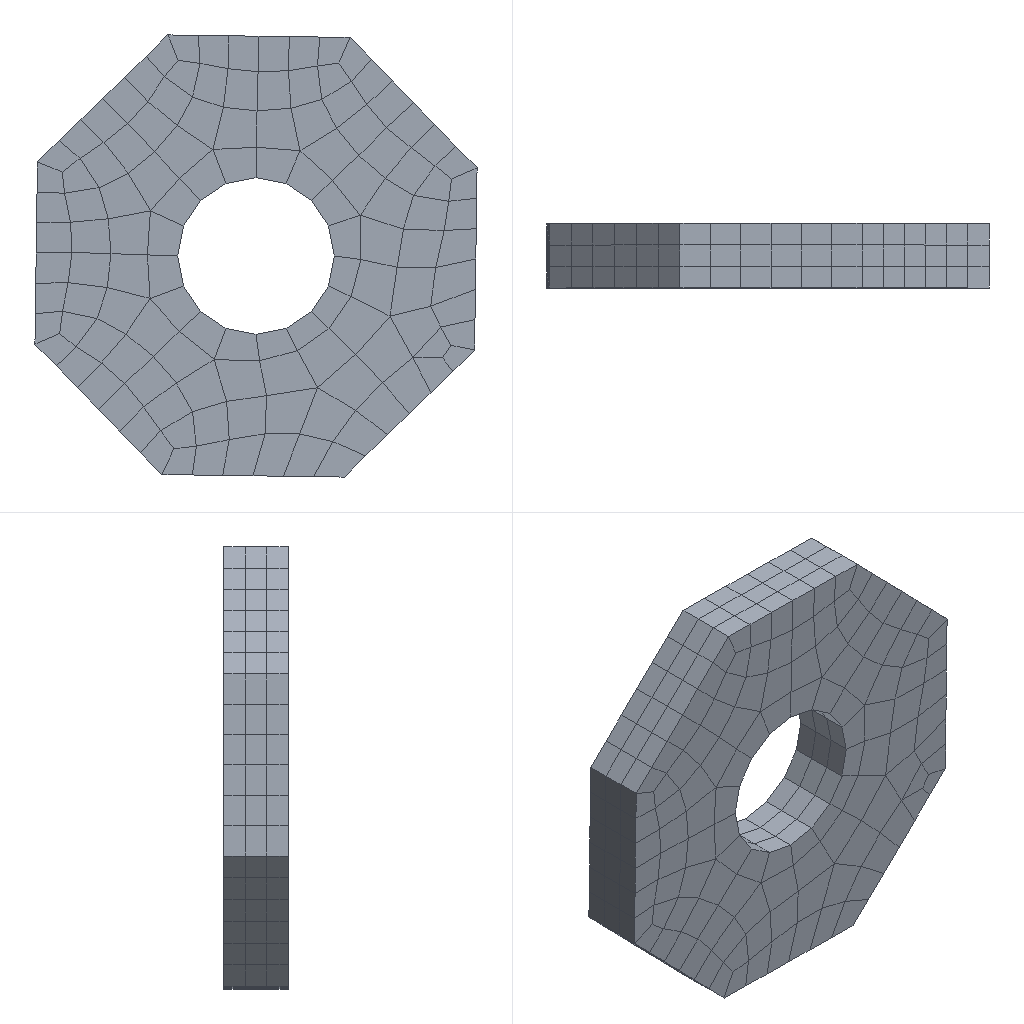Simulation study | ansys workbench
Ansys APDL input file, long lists of numbers shortened:
/batch
/config,noeldb,1     ! force off writing results to database
*get,_wallstrt,active,,time,wall
! ANSYS input file written by Workbench version 2022 R1
! File used for geometry attach: F:\ansys（分析文件汇总)\桥梁分析\平面.STEP
/title,__--____ (C5)
! ****** Begin Custom Load Command Snippet ******
/COM, ACT Extensions:
/COM,     LSDYNA, 2021.1
/COM,
! ****** End   Custom Load Command Snippet ******
*DIM,_wb_ProjectScratch_dir,string,248
_wb_ProjectScratch_dir(1) = 'F:\ansys（分析文件汇总)\桥梁分析\_ProjectScratch\ScrD469\'
*DIM,_wb_SolverFiles_dir,string,248
_wb_SolverFiles_dir(1) = 'F:\ansys（分析文件汇总)\桥梁分析\桥梁_files\dp0\SYS-2\MECH\'
*DIM,_wb_userfiles_dir,string,248
_wb_userfiles_dir(1) = 'F:\ansys（分析文件汇总)\桥梁分析\桥梁_files\user_files\'
/com,--- Data in consistent NMM units. See Solving Units in the help system for more information.
/units,MPA
/nopr
/wb,file,start              !  signify a WB generated input file
/prep7
! Turn off shape checking because checks already performed inside WB mesher.
! See help system for more information.
SHPP,OFF,,NOWARN
/nolist
etcon,set             ! allow ANSYS to choose best KEYOP's for 180x elements, resets any applicable keyopt to MAPDL defaults
/com,*********** Nodes for the whole assembly ***********
nblock,3,,2400
(1i9,3e20.9e3)
        1     1.551549580E+01     3.333333333E+00    -1.526301405E+01
! (2181 more lines like these left out)
-1
/wb,elem,start            !  set before creation of elements
/com,*********** Elements for Body 1 "__-FreeParts|__-__1" ***********
et,1,186
keyo,1,2,1          ! set full integration on SOLID186
eblock,19,solid,,366
(19i9)
        1        1        1        1        0        0        0        0       20        0        1        1       79       29       95      270      231      256      223
! (731 more lines like these left out)
-1
/wb,elem,end               !  done creating elements
/com,*********** Send User Defined Coordinate System(s) ***********
csys,0
toffst,273.15,  ! Temperature offset from absolute zero
/com,*********** Set Reference Temperature ***********
tref,22.
/wb,mat,start              !  starting to send materials
/com,*********** Send Materials ***********
Temperature = 'TEMP' ! Temperature
MP,DENS,1,7.85e-09,	! tonne mm^-3
MP,ALPX,1,1.2e-05,	! C^-1
MP,C,1,434000000,	! mm^2 s^-2 C^-1
MP,KXX,1,60.5,	! tonne mm s^-3 C^-1
MP,RSVX,1,0.00017,	! ohm mm
MP,EX,1,200000,	! tonne s^-2 mm^-1
MP,NUXY,1,0.3,
MP,MURX,1,10000,
/wb,mat,end                !  done sending materials
!************************* Model Summary ********************
!__-FreeParts|__-__1,	结构钢,	matid,	1
!************************* End Model Summary ********************
! get the diagonal of the bounding box. Needed later for other things
*get,_xmin,node,,mnloc,x
*get,_ymin,node,,mnloc,y
*get,_zmin,node,,mnloc,z
*get,_xmax,node,,mxloc,x
*get,_ymax,node,,mxloc,y
*get,_zmax,node,,mxloc,z
_ASMDIAG=(_xmax-_xmin)*(_xmax-_xmin)+(_ymax-_ymin)*(_ymax-_ymin)+(_zmax-_zmin)*(_zmax-_zmin)
_ASMDIAG=SQRT(_ASMDIAG)
/wb,contact,start          !  starting to send contact
/wb,contact,end            !  done creating contacts
/golist
/wb,load,start             !  starting to send loads
/com,*********** Fixed Supports ***********
CMBLOCK,_FIXEDSU,NODE,      430
(8i10)
       181       182       183       184       185       186       187       188
! (53 more lines like these left out)
cmsel,s,_FIXEDSU
d,all,all
nsel,all
/com,*********** Define Force Using Surface Effect Elements ***********
local,12,0,0.,0.,0.,0.,0.,0.
csys,0
et,2,154
eblock,10,,,48
(15i9)
      803        2        2        2       12      448      425      424      423     1865     1862     1860     1861
! (47 more lines like these left out)
-1
esel,s,type,,2
keyop,2,2,1                ! Apply load in local coordinate system
keyop,2,7,1                ! Use original area so load is constant in large deformation
esel,all
/gst,on,on
fini
*get,_numnode,node,0,count
*get,_numelem,elem,0,count
*get, _MAXELEMNUM, elem, 0, NUM, MAX
*get, _MAXNODENUM, node, 0, NUM, MAX
*get, _MAXELEMTYPE, etyp, 0, NUM, MAX
*get, _MAXREALCONST, real, 0, NUM, MAX
/go
/wb,load,end               !  done creating loads
/com,--- Number of total nodes = %_numnode%
/com,--- Number of contact elements = 48
/com,--- Number of spring elements = 0
/com,--- Number of bearing elements = 0
/com,--- Number of solid elements = 366
/com,--- Number of condensed parts = 0
/com,--- Number of total elements = %_numelem%
*get,_wallbsol,active,,time,wall
/com,****************************************************************************
/com,*************************    SOLUTION       ********************************
/com,****************************************************************************
/solu
antype,0                   ! static analysis
_thickRatio=  1     ! Ratio of thick parts in the model
eqsl,pcg,1e-8,,,,,,1
cntr,print,1               ! print out contact info and also make no initial contact an error
dmpoption,emat,no             ! Don't combine emat file for DANSYS
dmpoption,esav,no             ! Don't combine esav file for DANSYS
nldiag,cont,iter           ! print out contact info each equilibrium iteration
rescontrol,,none                 ! Do not keep any restart files
/com,****************************************************
/com,******************* SOLVE FOR LS 1 OF 1 ****************
esel,s,type,,2
nsle
sfe,all,1,pres,1,0.1216
sfe,all,2,pres,1,0.1216
sfe,all,3,pres,1,0.1216
nsel,all
esel,all
/nopr
/gopr
nsub,1,1,1
time,1.
outres,erase
outres,all,none
outres,nsol,all,
outres,rsol,all
outres,eangl,all
outres,etmp,all
outres,veng,all
outres,strs,all,
outres,epel,all,
outres,eppl,all,
outres,cont,all,
! *********** WB SOLVE COMMAND ***********
! check interactive state
*get,ANSINTER_,active,,int
*if,ANSINTER_,ne,0,then
/eof
*endif
solve
/com *************** Write FE CONNECTORS *********
CEWRITE,file,ce,,INTE
/com,****************************************************
/com,*************** FINISHED SOLVE FOR LS 1 *************
*get,_wallasol,active,,time,wall
/nopr
*get,_numnode,node,0,count
*get,_numelem,elem,0,count
*get, _MAXELEMNUM, elem, 0, NUM, MAX
*get, _MAXNODENUM, node, 0, NUM, MAX,,,INTERNAL
*get, _MAXELEMTYPE, etyp, 0, NUM, MAX
*get, _MAXREALCONST, real, 0, NUM, MAX
/gopr
*get,_PCGITER,active,,solu,cgiter
/post1
xmlo,ENCODING,ISO-8859-1
xmlo,parm
/xml,parm,xml
fini
/gopr
*get,_walldone,active,,time,wall
_preptime=(_wallbsol-_wallstrt)*3600
_solvtime=(_wallasol-_wallbsol)*3600
_posttime=(_walldone-_wallasol)*3600
_totaltim=(_walldone-_wallstrt)*3600
*get,_dlbratio,active,0,solu,dlbr
*get,_combtime,active,0,solu,comb
*get,_ssmode,active,0,solu,ssmm
*get,_ndofs,active,0,solu,ndof
*get,_sol_end_time,active,0,set,time
*if,_sol_end_time,eq,1.,then
/fclean				!clean distributed files
*endif
/com,--- Total number of nodes = %_numnode%
/com,--- Total number of elements = %_numelem%
/com,--- Element load balance ratio = %_dlbratio%
/com,--- Time to combine distributed files = %_combtime%
/com,--- Sparse memory mode = %_ssmode%
/com,--- Number of DOF = %_ndofs%
/wb,file,end               ! done with WB generated input